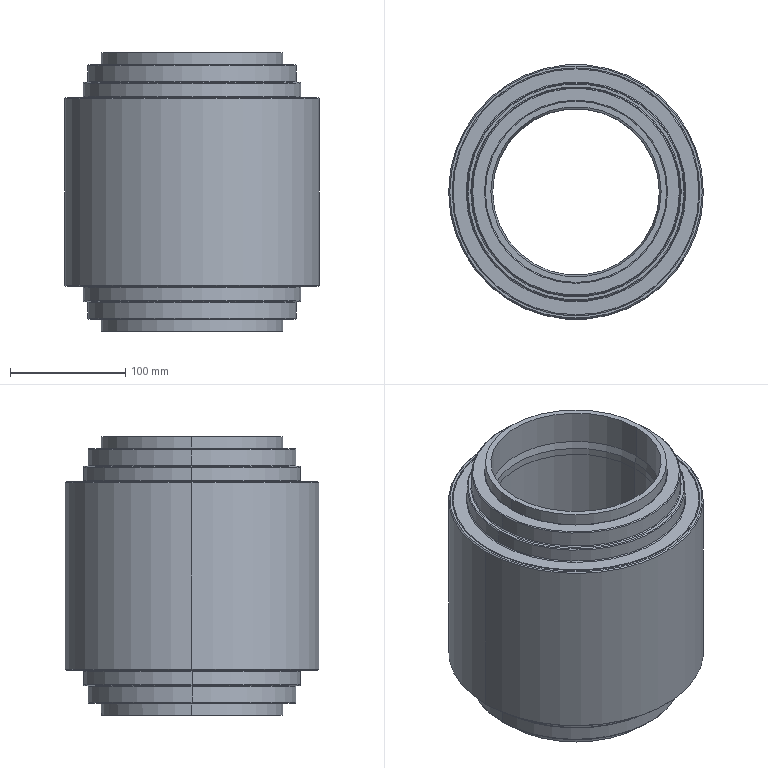Part | SolidWorks | features Revolution 12, CirPattern 2, Fillet 2, Chamfer 1, Cut 1 | 10 solids | 493 faces | box 220.662 x 220.662 x 241.2 mm | volume 3030333 mm3 | cone 260 | cylinder 125 | plane 84 | torus 24 | commonest cylinder face diameters 0.002 x52 157.15 x12 144.45 x10 177.77 x8 214.662 x8 147.6 x4